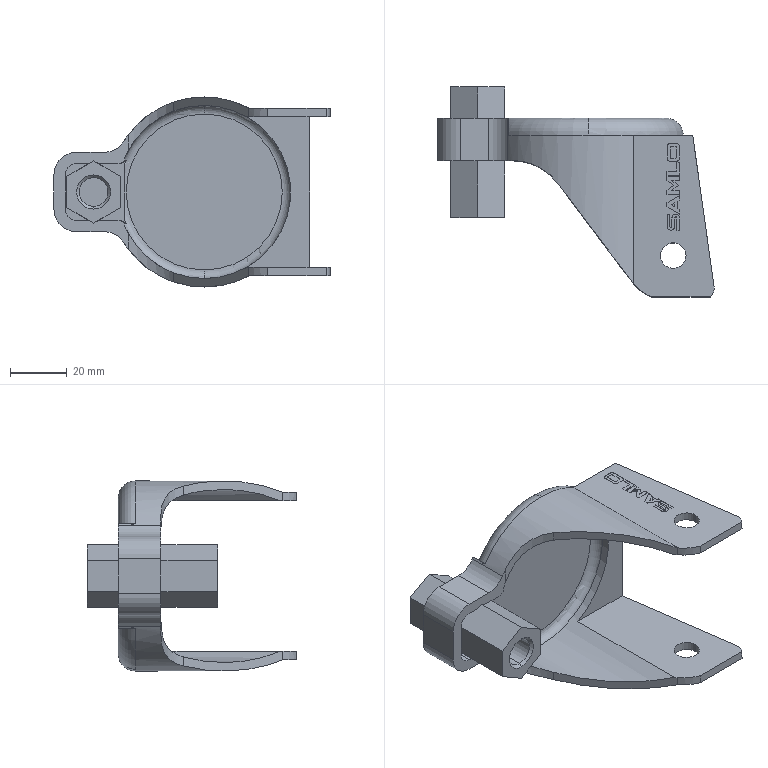Part | STEP file | JAJ-65_base | 1 solid | 139 faces | box 97.399 x 74 x 67.001 mm | volume 43204 mm3 | plane 96 | cylinder 35 | cone 4 | torus 4 | commonest cylinder face diameters 8 x6 1.037 x4 2.198 x4 9 x4 16 x4 0.743 x2